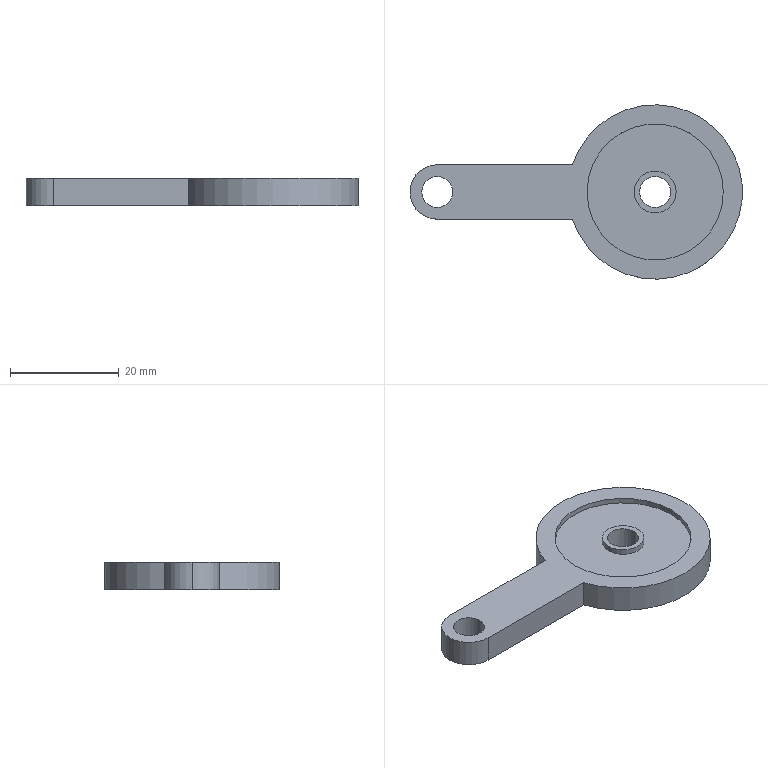Part | SolidWorks | features BaseBody 1, ICE 1 | 1 solid | 23 faces | box 61 x 32 x 5 mm | volume 4287 mm3 | cylinder 15 | plane 8 | commonest cylinder face diameters 5.7 x4 7.7 x4 25 x4 10 x2 32 x1
STEP:
#1=CARTESIAN_POINT('',(23.85,0.,2.5));
#2=VERTEX_POINT('',#1);
#3=CARTESIAN_POINT('',(16.15,0.,2.5));
#4=VERTEX_POINT('',#3);
#5=CARTESIAN_POINT('',(20.,0.,2.5));
#6=DIRECTION('',(0.,0.,1.));
#7=DIRECTION('',(1.,0.,0.));
#8=AXIS2_PLACEMENT_3D('',#5,#6,#7);
#9=CIRCLE('',#8,3.85);
#10=EDGE_CURVE('',#2,#4,#9,.T.);
#11=ORIENTED_EDGE('',*,*,#10,.F.);
#12=CARTESIAN_POINT('',(23.85,0.,1.5));
#13=VERTEX_POINT('',#12);
#14=CARTESIAN_POINT('',(23.85,0.,13.389));
#15=DIRECTION('',(0.,0.,-1.));
#16=VECTOR('',#15,1000.);
#17=LINE('',#14,#16);
#18=EDGE_CURVE('',#2,#13,#17,.T.);
#19=ORIENTED_EDGE('',*,*,#18,.T.);
#20=CARTESIAN_POINT('',(16.15,0.,1.5));
#21=VERTEX_POINT('',#20);
#22=CARTESIAN_POINT('',(20.,0.,1.5));
#23=DIRECTION('',(0.,0.,-1.));
#24=DIRECTION('',(1.,0.,0.));
#25=AXIS2_PLACEMENT_3D('',#22,#23,#24);
#26=CIRCLE('',#25,3.85);
#27=EDGE_CURVE('',#21,#13,#26,.T.);
#28=ORIENTED_EDGE('',*,*,#27,.F.);
#29=CARTESIAN_POINT('',(16.15,0.,13.389));
#30=DIRECTION('',(0.,0.,-1.));
#31=VECTOR('',#30,1000.);
#32=LINE('',#29,#31);
#33=EDGE_CURVE('',#4,#21,#32,.T.);
#34=ORIENTED_EDGE('',*,*,#33,.F.);
#35=EDGE_LOOP('',(#11,#19,#28,#34));
#36=FACE_OUTER_BOUND('',#35,.T.);
#37=CARTESIAN_POINT('',(20.,0.,13.389));
#38=DIRECTION('',(0.,0.,-1.));
#39=DIRECTION('',(-1.,0.,0.));
#40=AXIS2_PLACEMENT_3D('',#37,#38,#39);
#41=CYLINDRICAL_SURFACE('',#40,3.85);
#42=ADVANCED_FACE('',(#36),#41,.T.);
#43=CARTESIAN_POINT('',(17.15,0.,2.5));
#44=VERTEX_POINT('',#43);
#45=CARTESIAN_POINT('',(22.85,0.,2.5));
#46=VERTEX_POINT('',#45);
#47=CARTESIAN_POINT('',(20.,0.,2.5));
#48=DIRECTION('',(0.,0.,1.));
#49=DIRECTION('',(1.,0.,0.));
#50=AXIS2_PLACEMENT_3D('',#47,#48,#49);
#51=CIRCLE('',#50,2.85);
#52=EDGE_CURVE('',#44,#46,#51,.T.);
#53=ORIENTED_EDGE('',*,*,#52,.T.);
#54=CARTESIAN_POINT('',(22.85,0.,-2.5));
#55=VERTEX_POINT('',#54);
#56=CARTESIAN_POINT('',(22.85,0.,2.5));
#57=DIRECTION('',(0.,0.,-1.));
#58=VECTOR('',#57,1000.);
#59=LINE('',#56,#58);
#60=EDGE_CURVE('',#46,#55,#59,.T.);
#61=ORIENTED_EDGE('',*,*,#60,.T.);
#62=CARTESIAN_POINT('',(17.15,0.,-2.5));
#63=VERTEX_POINT('',#62);
#64=CARTESIAN_POINT('',(20.,0.,-2.5));
#65=DIRECTION('',(0.,0.,-1.));
#66=DIRECTION('',(1.,0.,0.));
#67=AXIS2_PLACEMENT_3D('',#64,#65,#66);
#68=CIRCLE('',#67,2.85);
#69=EDGE_CURVE('',#55,#63,#68,.T.);
#70=ORIENTED_EDGE('',*,*,#69,.T.);
#71=CARTESIAN_POINT('',(17.15,0.,2.5));
#72=DIRECTION('',(0.,0.,-1.));
#73=VECTOR('',#72,1000.);
#74=LINE('',#71,#73);
#75=EDGE_CURVE('',#44,#63,#74,.T.);
#76=ORIENTED_EDGE('',*,*,#75,.F.);
#77=EDGE_LOOP('',(#53,#61,#70,#76));
#78=FACE_OUTER_BOUND('',#77,.T.);
#79=CARTESIAN_POINT('',(20.,0.,2.5));
#80=DIRECTION('',(0.,0.,-1.));
#81=DIRECTION('',(-1.,0.,0.));
#82=AXIS2_PLACEMENT_3D('',#79,#80,#81);
#83=CYLINDRICAL_SURFACE('',#82,2.85);
#84=ADVANCED_FACE('',(#78),#83,.F.);
#85=CARTESIAN_POINT('',(16.15,0.,-1.5));
#86=VERTEX_POINT('',#85);
#87=CARTESIAN_POINT('',(23.85,0.,-1.5));
#88=VERTEX_POINT('',#87);
#89=CARTESIAN_POINT('',(20.,0.,-1.5));
#90=DIRECTION('',(0.,0.,-1.));
#91=DIRECTION('',(1.,0.,0.));
#92=AXIS2_PLACEMENT_3D('',#89,#90,#91);
#93=CIRCLE('',#92,3.85);
#94=EDGE_CURVE('',#86,#88,#93,.T.);
#95=ORIENTED_EDGE('',*,*,#94,.T.);
#96=CARTESIAN_POINT('',(23.85,0.,-2.5));
#97=VERTEX_POINT('',#96);
#98=CARTESIAN_POINT('',(23.85,0.,13.389));
#99=DIRECTION('',(0.,0.,-1.));
#100=VECTOR('',#99,1000.);
#101=LINE('',#98,#100);
#102=EDGE_CURVE('',#88,#97,#101,.T.);
#103=ORIENTED_EDGE('',*,*,#102,.T.);
#104=CARTESIAN_POINT('',(16.15,0.,-2.5));
#105=VERTEX_POINT('',#104);
#106=CARTESIAN_POINT('',(20.,0.,-2.5));
#107=DIRECTION('',(0.,0.,-1.));
#108=DIRECTION('',(1.,0.,0.));
#109=AXIS2_PLACEMENT_3D('',#106,#107,#108);
#110=CIRCLE('',#109,3.85);
#111=EDGE_CURVE('',#105,#97,#110,.T.);
#112=ORIENTED_EDGE('',*,*,#111,.F.);
#113=CARTESIAN_POINT('',(16.15,0.,13.389));
#114=DIRECTION('',(0.,0.,-1.));
#115=VECTOR('',#114,1000.);
#116=LINE('',#113,#115);
#117=EDGE_CURVE('',#86,#105,#116,.T.);
#118=ORIENTED_EDGE('',*,*,#117,.F.);
#119=EDGE_LOOP('',(#95,#103,#112,#118));
#120=FACE_OUTER_BOUND('',#119,.T.);
#121=CARTESIAN_POINT('',(20.,0.,13.389));
#122=DIRECTION('',(0.,0.,-1.));
#123=DIRECTION('',(-1.,0.,0.));
#124=AXIS2_PLACEMENT_3D('',#121,#122,#123);
#125=CYLINDRICAL_SURFACE('',#124,3.85);
#126=ADVANCED_FACE('',(#120),#125,.T.);
#127=CARTESIAN_POINT('',(7.5,0.,-1.5));
#128=VERTEX_POINT('',#127);
#129=CARTESIAN_POINT('',(32.5,0.,-1.5));
#130=VERTEX_POINT('',#129);
#131=CARTESIAN_POINT('',(20.,0.,-1.5));
#132=DIRECTION('',(0.,0.,1.));
#133=DIRECTION('',(1.,0.,0.));
#134=AXIS2_PLACEMENT_3D('',#131,#132,#133);
#135=CIRCLE('',#134,12.5);
#136=EDGE_CURVE('',#128,#130,#135,.T.);
#137=ORIENTED_EDGE('',*,*,#136,.T.);
#138=CARTESIAN_POINT('',(32.5,0.,-2.5));
#139=VERTEX_POINT('',#138);
#140=CARTESIAN_POINT('',(32.5,0.,-1.5));
#141=DIRECTION('',(0.,0.,-1.));
#142=VECTOR('',#141,1000.);
#143=LINE('',#140,#142);
#144=EDGE_CURVE('',#130,#139,#143,.T.);
#145=ORIENTED_EDGE('',*,*,#144,.T.);
#146=CARTESIAN_POINT('',(7.5,0.,-2.5));
#147=VERTEX_POINT('',#146);
#148=CARTESIAN_POINT('',(20.,0.,-2.5));
#149=DIRECTION('',(0.,0.,1.));
#150=DIRECTION('',(1.,0.,0.));
#151=AXIS2_PLACEMENT_3D('',#148,#149,#150);
#152=CIRCLE('',#151,12.5);
#153=EDGE_CURVE('',#147,#139,#152,.T.);
#154=ORIENTED_EDGE('',*,*,#153,.F.);
#155=CARTESIAN_POINT('',(7.5,0.,-1.5));
#156=DIRECTION('',(0.,0.,-1.));
#157=VECTOR('',#156,1000.);
#158=LINE('',#155,#157);
#159=EDGE_CURVE('',#128,#147,#158,.T.);
#160=ORIENTED_EDGE('',*,*,#159,.F.);
#161=EDGE_LOOP('',(#137,#145,#154,#160));
#162=FACE_OUTER_BOUND('',#161,.T.);
#163=CARTESIAN_POINT('',(20.,0.,-1.5));
#164=DIRECTION('',(0.,0.,-1.));
#165=DIRECTION('',(-1.,0.,0.));
#166=AXIS2_PLACEMENT_3D('',#163,#164,#165);
#167=CYLINDRICAL_SURFACE('',#166,12.5);
#168=ADVANCED_FACE('',(#162),#167,.F.);
#169=CARTESIAN_POINT('',(7.5,0.,1.5));
#170=VERTEX_POINT('',#169);
#171=CARTESIAN_POINT('',(32.5,0.,1.5));
#172=VERTEX_POINT('',#171);
#173=CARTESIAN_POINT('',(20.,0.,1.5));
#174=DIRECTION('',(0.,0.,1.));
#175=DIRECTION('',(1.,0.,0.));
#176=AXIS2_PLACEMENT_3D('',#173,#174,#175);
#177=CIRCLE('',#176,12.5);
#178=EDGE_CURVE('',#170,#172,#177,.T.);
#179=ORIENTED_EDGE('',*,*,#178,.F.);
#180=CARTESIAN_POINT('',(7.5,0.,2.5));
#181=VERTEX_POINT('',#180);
#182=CARTESIAN_POINT('',(7.5,0.,1.5));
#183=DIRECTION('',(0.,0.,1.));
#184=VECTOR('',#183,1000.);
#185=LINE('',#182,#184);
#186=EDGE_CURVE('',#170,#181,#185,.T.);
#187=ORIENTED_EDGE('',*,*,#186,.T.);
#188=CARTESIAN_POINT('',(32.5,0.,2.5));
#189=VERTEX_POINT('',#188);
#190=CARTESIAN_POINT('',(20.,0.,2.5));
#191=DIRECTION('',(0.,0.,1.));
#192=DIRECTION('',(1.,0.,0.));
#193=AXIS2_PLACEMENT_3D('',#190,#191,#192);
#194=CIRCLE('',#193,12.5);
#195=EDGE_CURVE('',#181,#189,#194,.T.);
#196=ORIENTED_EDGE('',*,*,#195,.T.);
#197=CARTESIAN_POINT('',(32.5,0.,1.5));
#198=DIRECTION('',(0.,0.,1.));
#199=VECTOR('',#198,1000.);
#200=LINE('',#197,#199);
#201=EDGE_CURVE('',#172,#189,#200,.T.);
#202=ORIENTED_EDGE('',*,*,#201,.F.);
#203=EDGE_LOOP('',(#179,#187,#196,#202));
#204=FACE_OUTER_BOUND('',#203,.T.);
#205=CARTESIAN_POINT('',(20.,0.,1.5));
#206=DIRECTION('',(0.,0.,1.));
#207=DIRECTION('',(1.,0.,0.));
#208=AXIS2_PLACEMENT_3D('',#205,#206,#207);
#209=CYLINDRICAL_SURFACE('',#208,12.5);
#210=ADVANCED_FACE('',(#204),#209,.F.);
#211=CARTESIAN_POINT('',(-22.85,0.,2.5));
#212=VERTEX_POINT('',#211);
#213=CARTESIAN_POINT('',(-17.15,0.,2.5));
#214=VERTEX_POINT('',#213);
#215=CARTESIAN_POINT('',(-20.,0.,2.5));
#216=DIRECTION('',(0.,0.,1.));
#217=DIRECTION('',(1.,0.,0.));
#218=AXIS2_PLACEMENT_3D('',#215,#216,#217);
#219=CIRCLE('',#218,2.85);
#220=EDGE_CURVE('',#212,#214,#219,.T.);
#221=ORIENTED_EDGE('',*,*,#220,.T.);
#222=CARTESIAN_POINT('',(-17.15,0.,-2.5));
#223=VERTEX_POINT('',#222);
#224=CARTESIAN_POINT('',(-17.15,0.,2.5));
#225=DIRECTION('',(0.,0.,-1.));
#226=VECTOR('',#225,1000.);
#227=LINE('',#224,#226);
#228=EDGE_CURVE('',#214,#223,#227,.T.);
#229=ORIENTED_EDGE('',*,*,#228,.T.);
#230=CARTESIAN_POINT('',(-22.85,0.,-2.5));
#231=VERTEX_POINT('',#230);
#232=CARTESIAN_POINT('',(-20.,0.,-2.5));
#233=DIRECTION('',(0.,0.,1.));
#234=DIRECTION('',(1.,0.,0.));
#235=AXIS2_PLACEMENT_3D('',#232,#233,#234);
#236=CIRCLE('',#235,2.85);
#237=EDGE_CURVE('',#231,#223,#236,.T.);
#238=ORIENTED_EDGE('',*,*,#237,.F.);
#239=CARTESIAN_POINT('',(-22.85,0.,2.5));
#240=DIRECTION('',(0.,0.,-1.));
#241=VECTOR('',#240,1000.);
#242=LINE('',#239,#241);
#243=EDGE_CURVE('',#212,#231,#242,.T.);
#244=ORIENTED_EDGE('',*,*,#243,.F.);
#245=EDGE_LOOP('',(#221,#229,#238,#244));
#246=FACE_OUTER_BOUND('',#245,.T.);
#247=CARTESIAN_POINT('',(-20.,0.,2.5));
#248=DIRECTION('',(0.,0.,-1.));
#249=DIRECTION('',(-1.,0.,0.));
#250=AXIS2_PLACEMENT_3D('',#247,#248,#249);
#251=CYLINDRICAL_SURFACE('',#250,2.85);
#252=ADVANCED_FACE('',(#246),#251,.F.);
#253=CARTESIAN_POINT('',(-25.,0.,2.5));
#254=VERTEX_POINT('',#253);
#255=CARTESIAN_POINT('',(-20.,-5.,2.5));
#256=VERTEX_POINT('',#255);
#257=CARTESIAN_POINT('',(-20.,0.,2.5));
#258=DIRECTION('',(0.,0.,1.));
#259=DIRECTION('',(1.,0.,0.));
#260=AXIS2_PLACEMENT_3D('',#257,#258,#259);
#261=CIRCLE('',#260,5.);
#262=EDGE_CURVE('',#254,#256,#261,.T.);
#263=ORIENTED_EDGE('',*,*,#262,.F.);
#264=CARTESIAN_POINT('',(-25.,0.,-2.5));
#265=VERTEX_POINT('',#264);
#266=CARTESIAN_POINT('',(-25.,0.,2.5));
#267=DIRECTION('',(0.,0.,-1.));
#268=VECTOR('',#267,1000.);
#269=LINE('',#266,#268);
#270=EDGE_CURVE('',#254,#265,#269,.T.);
#271=ORIENTED_EDGE('',*,*,#270,.T.);
#272=CARTESIAN_POINT('',(-20.,-5.,-2.5));
#273=VERTEX_POINT('',#272);
#274=CARTESIAN_POINT('',(-20.,0.,-2.5));
#275=DIRECTION('',(0.,0.,1.));
#276=DIRECTION('',(1.,0.,0.));
#277=AXIS2_PLACEMENT_3D('',#274,#275,#276);
#278=CIRCLE('',#277,5.);
#279=EDGE_CURVE('',#265,#273,#278,.T.);
#280=ORIENTED_EDGE('',*,*,#279,.T.);
#281=CARTESIAN_POINT('',(-20.,-5.,2.5));
#282=DIRECTION('',(0.,0.,-1.));
#283=VECTOR('',#282,1000.);
#284=LINE('',#281,#283);
#285=EDGE_CURVE('',#256,#273,#284,.T.);
#286=ORIENTED_EDGE('',*,*,#285,.F.);
#287=EDGE_LOOP('',(#263,#271,#280,#286));
#288=FACE_OUTER_BOUND('',#287,.T.);
#289=CARTESIAN_POINT('',(-20.,0.,2.5));
#290=DIRECTION('',(0.,0.,-1.));
#291=DIRECTION('',(-1.,0.,0.));
#292=AXIS2_PLACEMENT_3D('',#289,#290,#291);
#293=CYLINDRICAL_SURFACE('',#292,5.);
#294=ADVANCED_FACE('',(#288),#293,.T.);
#295=CARTESIAN_POINT('',(20.,0.,1.5));
#296=DIRECTION('',(0.,0.,1.));
#297=DIRECTION('',(1.,0.,0.));
#298=AXIS2_PLACEMENT_3D('',#295,#296,#297);
#299=CIRCLE('',#298,12.5);
#300=EDGE_CURVE('',#172,#170,#299,.T.);
#301=ORIENTED_EDGE('',*,*,#300,.T.);
#302=ORIENTED_EDGE('',*,*,#178,.T.);
#303=EDGE_LOOP('',(#301,#302));
#304=FACE_OUTER_BOUND('',#303,.T.);
#305=ORIENTED_EDGE('',*,*,#27,.T.);
#306=CARTESIAN_POINT('',(20.,0.,1.5));
#307=DIRECTION('',(0.,0.,-1.));
#308=DIRECTION('',(1.,0.,0.));
#309=AXIS2_PLACEMENT_3D('',#306,#307,#308);
#310=CIRCLE('',#309,3.85);
#311=EDGE_CURVE('',#13,#21,#310,.T.);
#312=ORIENTED_EDGE('',*,*,#311,.T.);
#313=EDGE_LOOP('',(#305,#312));
#314=FACE_BOUND('',#313,.T.);
#315=CARTESIAN_POINT('',(20.,0.,1.5));
#316=DIRECTION('',(0.,0.,1.));
#317=DIRECTION('',(1.,0.,0.));
#318=AXIS2_PLACEMENT_3D('',#315,#316,#317);
#319=PLANE('',#318);
#320=ADVANCED_FACE('',(#304,#314),#319,.T.);
#321=ORIENTED_EDGE('',*,*,#136,.F.);
#322=CARTESIAN_POINT('',(20.,0.,-1.5));
#323=DIRECTION('',(0.,0.,1.));
#324=DIRECTION('',(1.,0.,0.));
#325=AXIS2_PLACEMENT_3D('',#322,#323,#324);
#326=CIRCLE('',#325,12.5);
#327=EDGE_CURVE('',#130,#128,#326,.T.);
#328=ORIENTED_EDGE('',*,*,#327,.F.);
#329=EDGE_LOOP('',(#321,#328));
#330=FACE_OUTER_BOUND('',#329,.T.);
#331=ORIENTED_EDGE('',*,*,#94,.F.);
#332=CARTESIAN_POINT('',(20.,0.,-1.5));
#333=DIRECTION('',(0.,0.,-1.));
#334=DIRECTION('',(1.,0.,0.));
#335=AXIS2_PLACEMENT_3D('',#332,#333,#334);
#336=CIRCLE('',#335,3.85);
#337=EDGE_CURVE('',#88,#86,#336,.T.);
#338=ORIENTED_EDGE('',*,*,#337,.F.);
#339=EDGE_LOOP('',(#331,#338));
#340=FACE_BOUND('',#339,.T.);
#341=CARTESIAN_POINT('',(20.,0.,-1.5));
#342=DIRECTION('',(0.,0.,1.));
#343=DIRECTION('',(1.,0.,0.));
#344=AXIS2_PLACEMENT_3D('',#341,#342,#343);
#345=PLANE('',#344);
#346=ADVANCED_FACE('',(#330,#340),#345,.F.);
#347=CARTESIAN_POINT('',(4.801,-5.,2.5));
#348=VERTEX_POINT('',#347);
#349=CARTESIAN_POINT('',(4.801,-5.,-2.5));
#350=VERTEX_POINT('',#349);
#351=CARTESIAN_POINT('',(4.801,-5.,2.5));
#352=DIRECTION('',(0.,0.,-1.));
#353=VECTOR('',#352,1000.);
#354=LINE('',#351,#353);
#355=EDGE_CURVE('',#348,#350,#354,.T.);
#356=ORIENTED_EDGE('',*,*,#355,.F.);
#357=CARTESIAN_POINT('',(-20.,-5.,2.5));
#358=DIRECTION('',(1.,0.,0.));
#359=VECTOR('',#358,1000.);
#360=LINE('',#357,#359);
#361=EDGE_CURVE('',#256,#348,#360,.T.);
#362=ORIENTED_EDGE('',*,*,#361,.F.);
#363=ORIENTED_EDGE('',*,*,#285,.T.);
#364=CARTESIAN_POINT('',(-20.,-5.,-2.5));
#365=DIRECTION('',(1.,0.,0.));
#366=VECTOR('',#365,1000.);
#367=LINE('',#364,#366);
#368=EDGE_CURVE('',#273,#350,#367,.T.);
#369=ORIENTED_EDGE('',*,*,#368,.T.);
#370=EDGE_LOOP('',(#356,#362,#363,#369));
#371=FACE_OUTER_BOUND('',#370,.T.);
#372=CARTESIAN_POINT('',(-20.,-5.,2.5));
#373=DIRECTION('',(0.,1.,0.));
#374=DIRECTION('',(-1.,0.,0.));
#375=AXIS2_PLACEMENT_3D('',#372,#373,#374);
#376=PLANE('',#375);
#377=ADVANCED_FACE('',(#371),#376,.F.);
#378=CARTESIAN_POINT('',(4.801,5.,-2.5));
#379=VERTEX_POINT('',#378);
#380=CARTESIAN_POINT('',(4.801,5.,2.5));
#381=VERTEX_POINT('',#380);
#382=CARTESIAN_POINT('',(4.801,5.,2.5));
#383=DIRECTION('',(0.,0.,1.));
#384=VECTOR('',#383,1000.);
#385=LINE('',#382,#384);
#386=EDGE_CURVE('',#379,#381,#385,.T.);
#387=ORIENTED_EDGE('',*,*,#386,.F.);
#388=CARTESIAN_POINT('',(-20.,5.,-2.5));
#389=VERTEX_POINT('',#388);
#390=CARTESIAN_POINT('',(-20.,5.,-2.5));
#391=DIRECTION('',(-1.,0.,0.));
#392=VECTOR('',#391,1000.);
#393=LINE('',#390,#392);
#394=EDGE_CURVE('',#379,#389,#393,.T.);
#395=ORIENTED_EDGE('',*,*,#394,.T.);
#396=CARTESIAN_POINT('',(-20.,5.,2.5));
#397=VERTEX_POINT('',#396);
#398=CARTESIAN_POINT('',(-20.,5.,2.5));
#399=DIRECTION('',(0.,0.,-1.));
#400=VECTOR('',#399,1000.);
#401=LINE('',#398,#400);
#402=EDGE_CURVE('',#397,#389,#401,.T.);
#403=ORIENTED_EDGE('',*,*,#402,.F.);
#404=CARTESIAN_POINT('',(-20.,5.,2.5));
#405=DIRECTION('',(-1.,0.,0.));
#406=VECTOR('',#405,1000.);
#407=LINE('',#404,#406);
#408=EDGE_CURVE('',#381,#397,#407,.T.);
#409=ORIENTED_EDGE('',*,*,#408,.F.);
#410=EDGE_LOOP('',(#387,#395,#403,#409));
#411=FACE_OUTER_BOUND('',#410,.T.);
#412=CARTESIAN_POINT('',(-20.,5.,2.5));
#413=DIRECTION('',(0.,-1.,0.));
#414=DIRECTION('',(1.,0.,0.));
#415=AXIS2_PLACEMENT_3D('',#412,#413,#414);
#416=PLANE('',#415);
#417=ADVANCED_FACE('',(#411),#416,.F.);
#418=CARTESIAN_POINT('',(20.,0.,2.5));
#419=DIRECTION('',(0.,0.,1.));
#420=DIRECTION('',(1.,0.,0.));
#421=AXIS2_PLACEMENT_3D('',#418,#419,#420);
#422=CIRCLE('',#421,16.);
#423=EDGE_CURVE('',#348,#381,#422,.T.);
#424=ORIENTED_EDGE('',*,*,#423,.T.);
#425=ORIENTED_EDGE('',*,*,#408,.T.);
#426=CARTESIAN_POINT('',(-20.,0.,2.5));
#427=DIRECTION('',(0.,0.,1.));
#428=DIRECTION('',(1.,0.,0.));
#429=AXIS2_PLACEMENT_3D('',#426,#427,#428);
#430=CIRCLE('',#429,5.);
#431=EDGE_CURVE('',#397,#254,#430,.T.);
#432=ORIENTED_EDGE('',*,*,#431,.T.);
#433=ORIENTED_EDGE('',*,*,#262,.T.);
#434=ORIENTED_EDGE('',*,*,#361,.T.);
#435=EDGE_LOOP('',(#424,#425,#432,#433,#434));
#436=FACE_OUTER_BOUND('',#435,.T.);
#437=CARTESIAN_POINT('',(20.,0.,2.5));
#438=DIRECTION('',(0.,0.,1.));
#439=DIRECTION('',(1.,0.,0.));
#440=AXIS2_PLACEMENT_3D('',#437,#438,#439);
#441=CIRCLE('',#440,12.5);
#442=EDGE_CURVE('',#189,#181,#441,.T.);
#443=ORIENTED_EDGE('',*,*,#442,.F.);
#444=ORIENTED_EDGE('',*,*,#195,.F.);
#445=EDGE_LOOP('',(#443,#444));
#446=FACE_BOUND('',#445,.T.);
#447=ORIENTED_EDGE('',*,*,#220,.F.);
#448=CARTESIAN_POINT('',(-20.,0.,2.5));
#449=DIRECTION('',(0.,0.,1.));
#450=DIRECTION('',(1.,0.,0.));
#451=AXIS2_PLACEMENT_3D('',#448,#449,#450);
#452=CIRCLE('',#451,2.85);
#453=EDGE_CURVE('',#214,#212,#452,.T.);
#454=ORIENTED_EDGE('',*,*,#453,.F.);
#455=EDGE_LOOP('',(#447,#454));
#456=FACE_BOUND('',#455,.T.);
#457=CARTESIAN_POINT('',(-20.,0.,2.5));
#458=DIRECTION('',(0.,0.,1.));
#459=DIRECTION('',(1.,0.,0.));
#460=AXIS2_PLACEMENT_3D('',#457,#458,#459);
#461=PLANE('',#460);
#462=ADVANCED_FACE('',(#436,#446,#456),#461,.T.);
#463=ORIENTED_EDGE('',*,*,#153,.T.);
#464=CARTESIAN_POINT('',(20.,0.,-2.5));
#465=DIRECTION('',(0.,0.,1.));
#466=DIRECTION('',(1.,0.,0.));
#467=AXIS2_PLACEMENT_3D('',#464,#465,#466);
#468=CIRCLE('',#467,12.5);
#469=EDGE_CURVE('',#139,#147,#468,.T.);
#470=ORIENTED_EDGE('',*,*,#469,.T.);
#471=EDGE_LOOP('',(#463,#470));
#472=FACE_BOUND('',#471,.T.);
#473=ORIENTED_EDGE('',*,*,#394,.F.);
#474=CARTESIAN_POINT('',(20.,0.,-2.5));
#475=DIRECTION('',(0.,0.,1.));
#476=DIRECTION('',(1.,0.,0.));
#477=AXIS2_PLACEMENT_3D('',#474,#475,#476);
#478=CIRCLE('',#477,16.);
#479=EDGE_CURVE('',#350,#379,#478,.T.);
#480=ORIENTED_EDGE('',*,*,#479,.F.);
#481=ORIENTED_EDGE('',*,*,#368,.F.);
#482=ORIENTED_EDGE('',*,*,#279,.F.);
#483=CARTESIAN_POINT('',(-20.,0.,-2.5));
#484=DIRECTION('',(0.,0.,1.));
#485=DIRECTION('',(1.,0.,0.));
#486=AXIS2_PLACEMENT_3D('',#483,#484,#485);
#487=CIRCLE('',#486,5.);
#488=EDGE_CURVE('',#389,#265,#487,.T.);
#489=ORIENTED_EDGE('',*,*,#488,.F.);
#490=EDGE_LOOP('',(#473,#480,#481,#482,#489));
#491=FACE_OUTER_BOUND('',#490,.T.);
#492=ORIENTED_EDGE('',*,*,#237,.T.);
#493=CARTESIAN_POINT('',(-20.,0.,-2.5));
#494=DIRECTION('',(0.,0.,1.));
#495=DIRECTION('',(1.,0.,0.));
#496=AXIS2_PLACEMENT_3D('',#493,#494,#495);
#497=CIRCLE('',#496,2.85);
#498=EDGE_CURVE('',#223,#231,#497,.T.);
#499=ORIENTED_EDGE('',*,*,#498,.T.);
#500=EDGE_LOOP('',(#492,#499));
#501=FACE_BOUND('',#500,.T.);
#502=CARTESIAN_POINT('',(-20.,0.,-2.5));
#503=DIRECTION('',(0.,0.,1.));
#504=DIRECTION('',(1.,0.,0.));
#505=AXIS2_PLACEMENT_3D('',#502,#503,#504);
#506=PLANE('',#505);
#507=ADVANCED_FACE('',(#472,#491,#501),#506,.F.);
#508=ORIENTED_EDGE('',*,*,#270,.F.);
#509=ORIENTED_EDGE('',*,*,#431,.F.);
#510=ORIENTED_EDGE('',*,*,#402,.T.);
#511=ORIENTED_EDGE('',*,*,#488,.T.);
#512=EDGE_LOOP('',(#508,#509,#510,#511));
#513=FACE_OUTER_BOUND('',#512,.T.);
#514=CARTESIAN_POINT('',(-20.,0.,2.5));
#515=DIRECTION('',(0.,0.,-1.));
#516=DIRECTION('',(-1.,0.,0.));
#517=AXIS2_PLACEMENT_3D('',#514,#515,#516);
#518=CYLINDRICAL_SURFACE('',#517,5.);
#519=ADVANCED_FACE('',(#513),#518,.T.);
#520=ORIENTED_EDGE('',*,*,#228,.F.);
#521=ORIENTED_EDGE('',*,*,#453,.T.);
#522=ORIENTED_EDGE('',*,*,#243,.T.);
#523=ORIENTED_EDGE('',*,*,#498,.F.);
#524=EDGE_LOOP('',(#520,#521,#522,#523));
#525=FACE_OUTER_BOUND('',#524,.T.);
#526=CARTESIAN_POINT('',(-20.,0.,2.5));
#527=DIRECTION('',(0.,0.,-1.));
#528=DIRECTION('',(-1.,0.,0.));
#529=AXIS2_PLACEMENT_3D('',#526,#527,#528);
#530=CYLINDRICAL_SURFACE('',#529,2.85);
#531=ADVANCED_FACE('',(#525),#530,.F.);
#532=ORIENTED_EDGE('',*,*,#479,.T.);
#533=ORIENTED_EDGE('',*,*,#386,.T.);
#534=ORIENTED_EDGE('',*,*,#423,.F.);
#535=ORIENTED_EDGE('',*,*,#355,.T.);
#536=EDGE_LOOP('',(#532,#533,#534,#535));
#537=FACE_OUTER_BOUND('',#536,.T.);
#538=CARTESIAN_POINT('',(20.,0.,2.5));
#539=DIRECTION('',(0.,0.,-1.));
#540=DIRECTION('',(-1.,0.,0.));
#541=AXIS2_PLACEMENT_3D('',#538,#539,#540);
#542=CYLINDRICAL_SURFACE('',#541,16.);
#543=ADVANCED_FACE('',(#537),#542,.T.);
#544=ORIENTED_EDGE('',*,*,#186,.F.);
#545=ORIENTED_EDGE('',*,*,#300,.F.);
#546=ORIENTED_EDGE('',*,*,#201,.T.);
#547=ORIENTED_EDGE('',*,*,#442,.T.);
#548=EDGE_LOOP('',(#544,#545,#546,#547));
#549=FACE_OUTER_BOUND('',#548,.T.);
#550=CARTESIAN_POINT('',(20.,0.,1.5));
#551=DIRECTION('',(0.,0.,1.));
#552=DIRECTION('',(1.,0.,0.));
#553=AXIS2_PLACEMENT_3D('',#550,#551,#552);
#554=CYLINDRICAL_SURFACE('',#553,12.5);
#555=ADVANCED_FACE('',(#549),#554,.F.);
#556=ORIENTED_EDGE('',*,*,#144,.F.);
#557=ORIENTED_EDGE('',*,*,#327,.T.);
#558=ORIENTED_EDGE('',*,*,#159,.T.);
#559=ORIENTED_EDGE('',*,*,#469,.F.);
#560=EDGE_LOOP('',(#556,#557,#558,#559));
#561=FACE_OUTER_BOUND('',#560,.T.);
#562=CARTESIAN_POINT('',(20.,0.,-1.5));
#563=DIRECTION('',(0.,0.,-1.));
#564=DIRECTION('',(-1.,0.,0.));
#565=AXIS2_PLACEMENT_3D('',#562,#563,#564);
#566=CYLINDRICAL_SURFACE('',#565,12.5);
#567=ADVANCED_FACE('',(#561),#566,.F.);
#568=ORIENTED_EDGE('',*,*,#102,.F.);
#569=ORIENTED_EDGE('',*,*,#337,.T.);
#570=ORIENTED_EDGE('',*,*,#117,.T.);
#571=CARTESIAN_POINT('',(20.,0.,-2.5));
#572=DIRECTION('',(0.,0.,-1.));
#573=DIRECTION('',(1.,0.,0.));
#574=AXIS2_PLACEMENT_3D('',#571,#572,#573);
#575=CIRCLE('',#574,3.85);
#576=EDGE_CURVE('',#97,#105,#575,.T.);
#577=ORIENTED_EDGE('',*,*,#576,.F.);
#578=EDGE_LOOP('',(#568,#569,#570,#577));
#579=FACE_OUTER_BOUND('',#578,.T.);
#580=CARTESIAN_POINT('',(20.,0.,13.389));
#581=DIRECTION('',(0.,0.,-1.));
#582=DIRECTION('',(-1.,0.,0.));
#583=AXIS2_PLACEMENT_3D('',#580,#581,#582);
#584=CYLINDRICAL_SURFACE('',#583,3.85);
#585=ADVANCED_FACE('',(#579),#584,.T.);
#586=ORIENTED_EDGE('',*,*,#111,.T.);
#587=ORIENTED_EDGE('',*,*,#576,.T.);
#588=EDGE_LOOP('',(#586,#587));
#589=FACE_OUTER_BOUND('',#588,.T.);
#590=CARTESIAN_POINT('',(20.,0.,-2.5));
#591=DIRECTION('',(0.,0.,-1.));
#592=DIRECTION('',(1.,0.,0.));
#593=AXIS2_PLACEMENT_3D('',#590,#591,#592);
#594=CIRCLE('',#593,2.85);
#595=EDGE_CURVE('',#63,#55,#594,.T.);
#596=ORIENTED_EDGE('',*,*,#595,.F.);
#597=ORIENTED_EDGE('',*,*,#69,.F.);
#598=EDGE_LOOP('',(#596,#597));
#599=FACE_BOUND('',#598,.T.);
#600=CARTESIAN_POINT('',(-20.,0.,-2.5));
#601=DIRECTION('',(0.,0.,1.));
#602=DIRECTION('',(1.,0.,0.));
#603=AXIS2_PLACEMENT_3D('',#600,#601,#602);
#604=PLANE('',#603);
#605=ADVANCED_FACE('',(#589,#599),#604,.F.);
#606=ORIENTED_EDGE('',*,*,#60,.F.);
#607=CARTESIAN_POINT('',(20.,0.,2.5));
#608=DIRECTION('',(0.,0.,1.));
#609=DIRECTION('',(1.,0.,0.));
#610=AXIS2_PLACEMENT_3D('',#607,#608,#609);
#611=CIRCLE('',#610,2.85);
#612=EDGE_CURVE('',#46,#44,#611,.T.);
#613=ORIENTED_EDGE('',*,*,#612,.T.);
#614=ORIENTED_EDGE('',*,*,#75,.T.);
#615=ORIENTED_EDGE('',*,*,#595,.T.);
#616=EDGE_LOOP('',(#606,#613,#614,#615));
#617=FACE_OUTER_BOUND('',#616,.T.);
#618=CARTESIAN_POINT('',(20.,0.,2.5));
#619=DIRECTION('',(0.,0.,-1.));
#620=DIRECTION('',(-1.,0.,0.));
#621=AXIS2_PLACEMENT_3D('',#618,#619,#620);
#622=CYLINDRICAL_SURFACE('',#621,2.85);
#623=ADVANCED_FACE('',(#617),#622,.F.);
#624=ORIENTED_EDGE('',*,*,#18,.F.);
#625=CARTESIAN_POINT('',(20.,0.,2.5));
#626=DIRECTION('',(0.,0.,1.));
#627=DIRECTION('',(1.,0.,0.));
#628=AXIS2_PLACEMENT_3D('',#625,#626,#627);
#629=CIRCLE('',#628,3.85);
#630=EDGE_CURVE('',#4,#2,#629,.T.);
#631=ORIENTED_EDGE('',*,*,#630,.F.);
#632=ORIENTED_EDGE('',*,*,#33,.T.);
#633=ORIENTED_EDGE('',*,*,#311,.F.);
#634=EDGE_LOOP('',(#624,#631,#632,#633));
#635=FACE_OUTER_BOUND('',#634,.T.);
#636=CARTESIAN_POINT('',(20.,0.,13.389));
#637=DIRECTION('',(0.,0.,-1.));
#638=DIRECTION('',(-1.,0.,0.));
#639=AXIS2_PLACEMENT_3D('',#636,#637,#638);
#640=CYLINDRICAL_SURFACE('',#639,3.85);
#641=ADVANCED_FACE('',(#635),#640,.T.);
#642=ORIENTED_EDGE('',*,*,#52,.F.);
#643=ORIENTED_EDGE('',*,*,#612,.F.);
#644=EDGE_LOOP('',(#642,#643));
#645=FACE_BOUND('',#644,.T.);
#646=ORIENTED_EDGE('',*,*,#630,.T.);
#647=ORIENTED_EDGE('',*,*,#10,.T.);
#648=EDGE_LOOP('',(#646,#647));
#649=FACE_OUTER_BOUND('',#648,.T.);
#650=CARTESIAN_POINT('',(-20.,0.,2.5));
#651=DIRECTION('',(0.,0.,1.));
#652=DIRECTION('',(1.,0.,0.));
#653=AXIS2_PLACEMENT_3D('',#650,#651,#652);
#654=PLANE('',#653);
#655=ADVANCED_FACE('',(#645,#649),#654,.T.);
#656=CLOSED_SHELL('',(#42,#84,#126,#168,#210,#252,#294,#320,#346,#377,#417,#462,#507,#519,#531,#543,#555,#567,#585,#605,#623,#641,#655));
#657=MANIFOLD_SOLID_BREP('',#656);
#658=CARTESIAN_POINT('',(0.,0.,0.));
#659=DIRECTION('',(0.,0.,1.));
#660=DIRECTION('',(1.,0.,0.));
#661=AXIS2_PLACEMENT_3D('',#658,#659,#660);
#662=(LENGTH_UNIT()NAMED_UNIT(*)SI_UNIT(.MILLI.,.METRE.));
#663=UNCERTAINTY_MEASURE_WITH_UNIT(LENGTH_MEASURE(0.00001),#662,'','');
#664=(NAMED_UNIT(*)PLANE_ANGLE_UNIT()SI_UNIT($,.RADIAN.));
#665=(NAMED_UNIT(*)SI_UNIT($,.STERADIAN.)SOLID_ANGLE_UNIT());
#666=(GEOMETRIC_REPRESENTATION_CONTEXT(3)GLOBAL_UNCERTAINTY_ASSIGNED_CONTEXT((#663))GLOBAL_UNIT_ASSIGNED_CONTEXT((#662,#664,#665))REPRESENTATION_CONTEXT('',''));
#667=ADVANCED_BREP_SHAPE_REPRESENTATION('',(#657,#661),#666);